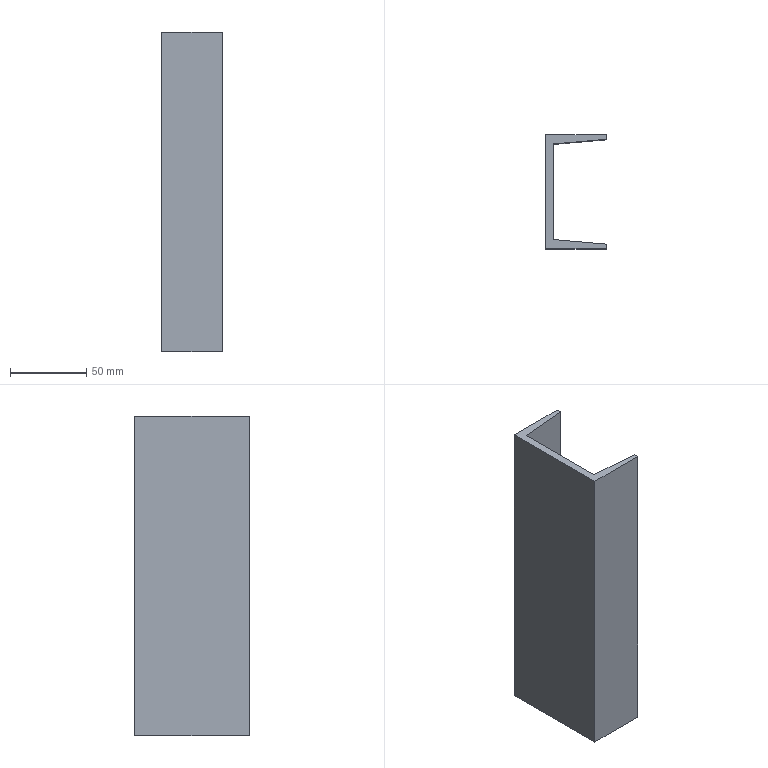Part | STEP file | BCC3 H13_7 | 1 solid | 10 faces | box 40 x 75 x 210 mm | volume 145356 mm3 | plane 10
STEP:
#1=CARTESIAN_POINT('',(0.,0.,0.));
#2=DIRECTION('',(0.,0.,1.));
#3=DIRECTION('',(1.,0.,0.));
#4=AXIS2_PLACEMENT_3D('',#1,#2,#3);
#5=CARTESIAN_POINT('',(40.,37.5,-105.));
#6=VERTEX_POINT('',#5);
#7=CARTESIAN_POINT('',(0.,37.5,-105.));
#8=VERTEX_POINT('',#7);
#9=CARTESIAN_POINT('',(40.,37.5,-105.));
#10=DIRECTION('',(-1.,0.,0.));
#11=VECTOR('',#10,1.);
#12=LINE('',#9,#11);
#13=CARTESIAN_POINT('',(40.,37.5,105.));
#14=DIRECTION('',(0.,-1.,0.));
#15=DIRECTION('',(0.,0.,-1.));
#16=AXIS2_PLACEMENT_3D('',#13,#14,#15);
#17=PLANE('',#16);
#18=CARTESIAN_POINT('',(210.,0.));
#19=DIRECTION('',(0.,-1.));
#20=VECTOR('',#19,1.);
#21=LINE('',#18,#20);
#22=(GEOMETRIC_REPRESENTATION_CONTEXT(2)PARAMETRIC_REPRESENTATION_CONTEXT()REPRESENTATION_CONTEXT('',''));
#23=DEFINITIONAL_REPRESENTATION('',(#21),#22);
#24=PCURVE('',#17,#23);
#25=CARTESIAN_POINT('',(0.,0.,-105.));
#26=DIRECTION('',(0.,0.,1.));
#27=DIRECTION('',(1.,0.,0.));
#28=AXIS2_PLACEMENT_3D('',#25,#26,#27);
#29=PLANE('',#28);
#30=CARTESIAN_POINT('',(40.,37.5));
#31=DIRECTION('',(-1.,0.));
#32=VECTOR('',#31,1.);
#33=LINE('',#30,#32);
#34=(GEOMETRIC_REPRESENTATION_CONTEXT(2)PARAMETRIC_REPRESENTATION_CONTEXT()REPRESENTATION_CONTEXT('',''));
#35=DEFINITIONAL_REPRESENTATION('',(#33),#34);
#36=PCURVE('',#29,#35);
#37=SURFACE_CURVE('',#12,(#24,#36),.PCURVE_S1.);
#38=EDGE_CURVE('',#6,#8,#37,.T.);
#39=ORIENTED_EDGE('',*,*,#38,.T.);
#40=CARTESIAN_POINT('',(0.,37.5,105.));
#41=VERTEX_POINT('',#40);
#42=CARTESIAN_POINT('',(0.,37.5,105.));
#43=DIRECTION('',(0.,0.,-1.));
#44=VECTOR('',#43,1.);
#45=LINE('',#42,#44);
#46=CARTESIAN_POINT('',(0.,-40.));
#47=DIRECTION('',(1.,0.));
#48=VECTOR('',#47,1.);
#49=LINE('',#46,#48);
#50=(GEOMETRIC_REPRESENTATION_CONTEXT(2)PARAMETRIC_REPRESENTATION_CONTEXT()REPRESENTATION_CONTEXT('',''));
#51=DEFINITIONAL_REPRESENTATION('',(#49),#50);
#52=PCURVE('',#17,#51);
#53=CARTESIAN_POINT('',(0.,37.5,105.));
#54=DIRECTION('',(1.,0.,0.));
#55=DIRECTION('',(0.,0.,-1.));
#56=AXIS2_PLACEMENT_3D('',#53,#54,#55);
#57=PLANE('',#56);
#58=CARTESIAN_POINT('',(0.,0.));
#59=DIRECTION('',(1.,0.));
#60=VECTOR('',#59,1.);
#61=LINE('',#58,#60);
#62=(GEOMETRIC_REPRESENTATION_CONTEXT(2)PARAMETRIC_REPRESENTATION_CONTEXT()REPRESENTATION_CONTEXT('',''));
#63=DEFINITIONAL_REPRESENTATION('',(#61),#62);
#64=PCURVE('',#57,#63);
#65=SURFACE_CURVE('',#45,(#52,#64),.PCURVE_S1.);
#66=EDGE_CURVE('',#41,#8,#65,.T.);
#67=ORIENTED_EDGE('',*,*,#66,.F.);
#68=CARTESIAN_POINT('',(40.,37.5,105.));
#69=VERTEX_POINT('',#68);
#70=CARTESIAN_POINT('',(40.,37.5,105.));
#71=DIRECTION('',(-1.,0.,0.));
#72=VECTOR('',#71,1.);
#73=LINE('',#70,#72);
#74=CARTESIAN_POINT('',(0.,0.));
#75=DIRECTION('',(0.,-1.));
#76=VECTOR('',#75,1.);
#77=LINE('',#74,#76);
#78=(GEOMETRIC_REPRESENTATION_CONTEXT(2)PARAMETRIC_REPRESENTATION_CONTEXT()REPRESENTATION_CONTEXT('',''));
#79=DEFINITIONAL_REPRESENTATION('',(#77),#78);
#80=PCURVE('',#17,#79);
#81=CARTESIAN_POINT('',(0.,0.,105.));
#82=DIRECTION('',(0.,0.,1.));
#83=DIRECTION('',(1.,0.,0.));
#84=AXIS2_PLACEMENT_3D('',#81,#82,#83);
#85=PLANE('',#84);
#86=CARTESIAN_POINT('',(40.,37.5));
#87=DIRECTION('',(-1.,0.));
#88=VECTOR('',#87,1.);
#89=LINE('',#86,#88);
#90=(GEOMETRIC_REPRESENTATION_CONTEXT(2)PARAMETRIC_REPRESENTATION_CONTEXT()REPRESENTATION_CONTEXT('',''));
#91=DEFINITIONAL_REPRESENTATION('',(#89),#90);
#92=PCURVE('',#85,#91);
#93=SURFACE_CURVE('',#73,(#80,#92),.PCURVE_S1.);
#94=EDGE_CURVE('',#69,#41,#93,.T.);
#95=ORIENTED_EDGE('',*,*,#94,.F.);
#96=CARTESIAN_POINT('',(40.,37.5,105.));
#97=DIRECTION('',(0.,0.,-1.));
#98=VECTOR('',#97,1.);
#99=LINE('',#96,#98);
#100=CARTESIAN_POINT('',(0.,0.));
#101=DIRECTION('',(1.,0.));
#102=VECTOR('',#101,1.);
#103=LINE('',#100,#102);
#104=(GEOMETRIC_REPRESENTATION_CONTEXT(2)PARAMETRIC_REPRESENTATION_CONTEXT()REPRESENTATION_CONTEXT('',''));
#105=DEFINITIONAL_REPRESENTATION('',(#103),#104);
#106=PCURVE('',#17,#105);
#107=CARTESIAN_POINT('',(40.,34.5,105.));
#108=DIRECTION('',(-1.,0.,0.));
#109=DIRECTION('',(0.,0.,1.));
#110=AXIS2_PLACEMENT_3D('',#107,#108,#109);
#111=PLANE('',#110);
#112=CARTESIAN_POINT('',(0.,3.));
#113=DIRECTION('',(-1.,0.));
#114=VECTOR('',#113,1.);
#115=LINE('',#112,#114);
#116=(GEOMETRIC_REPRESENTATION_CONTEXT(2)PARAMETRIC_REPRESENTATION_CONTEXT()REPRESENTATION_CONTEXT('',''));
#117=DEFINITIONAL_REPRESENTATION('',(#115),#116);
#118=PCURVE('',#111,#117);
#119=SURFACE_CURVE('',#99,(#106,#118),.PCURVE_S1.);
#120=EDGE_CURVE('',#69,#6,#119,.T.);
#121=ORIENTED_EDGE('',*,*,#120,.T.);
#122=EDGE_LOOP('',(#39,#67,#95,#121));
#123=FACE_BOUND('',#122,.T.);
#124=ADVANCED_FACE('',(#123),#17,.F.);
#125=CARTESIAN_POINT('',(0.,-37.5,-105.));
#126=VERTEX_POINT('',#125);
#127=CARTESIAN_POINT('',(0.,37.5,-105.));
#128=DIRECTION('',(0.,-1.,0.));
#129=VECTOR('',#128,1.);
#130=LINE('',#127,#129);
#131=CARTESIAN_POINT('',(210.,0.));
#132=DIRECTION('',(0.,-1.));
#133=VECTOR('',#132,1.);
#134=LINE('',#131,#133);
#135=(GEOMETRIC_REPRESENTATION_CONTEXT(2)PARAMETRIC_REPRESENTATION_CONTEXT()REPRESENTATION_CONTEXT('',''));
#136=DEFINITIONAL_REPRESENTATION('',(#134),#135);
#137=PCURVE('',#57,#136);
#138=CARTESIAN_POINT('',(0.,37.5));
#139=DIRECTION('',(0.,-1.));
#140=VECTOR('',#139,1.);
#141=LINE('',#138,#140);
#142=(GEOMETRIC_REPRESENTATION_CONTEXT(2)PARAMETRIC_REPRESENTATION_CONTEXT()REPRESENTATION_CONTEXT('',''));
#143=DEFINITIONAL_REPRESENTATION('',(#141),#142);
#144=PCURVE('',#29,#143);
#145=SURFACE_CURVE('',#130,(#137,#144),.PCURVE_S1.);
#146=EDGE_CURVE('',#8,#126,#145,.T.);
#147=ORIENTED_EDGE('',*,*,#146,.T.);
#148=CARTESIAN_POINT('',(0.,-37.5,105.));
#149=VERTEX_POINT('',#148);
#150=CARTESIAN_POINT('',(0.,-37.5,105.));
#151=DIRECTION('',(0.,0.,-1.));
#152=VECTOR('',#151,1.);
#153=LINE('',#150,#152);
#154=CARTESIAN_POINT('',(0.,-75.));
#155=DIRECTION('',(1.,0.));
#156=VECTOR('',#155,1.);
#157=LINE('',#154,#156);
#158=(GEOMETRIC_REPRESENTATION_CONTEXT(2)PARAMETRIC_REPRESENTATION_CONTEXT()REPRESENTATION_CONTEXT('',''));
#159=DEFINITIONAL_REPRESENTATION('',(#157),#158);
#160=PCURVE('',#57,#159);
#161=CARTESIAN_POINT('',(0.,-37.5,105.));
#162=DIRECTION('',(0.,1.,0.));
#163=DIRECTION('',(0.,0.,1.));
#164=AXIS2_PLACEMENT_3D('',#161,#162,#163);
#165=PLANE('',#164);
#166=CARTESIAN_POINT('',(0.,0.));
#167=DIRECTION('',(-1.,0.));
#168=VECTOR('',#167,1.);
#169=LINE('',#166,#168);
#170=(GEOMETRIC_REPRESENTATION_CONTEXT(2)PARAMETRIC_REPRESENTATION_CONTEXT()REPRESENTATION_CONTEXT('',''));
#171=DEFINITIONAL_REPRESENTATION('',(#169),#170);
#172=PCURVE('',#165,#171);
#173=SURFACE_CURVE('',#153,(#160,#172),.PCURVE_S1.);
#174=EDGE_CURVE('',#149,#126,#173,.T.);
#175=ORIENTED_EDGE('',*,*,#174,.F.);
#176=CARTESIAN_POINT('',(0.,37.5,105.));
#177=DIRECTION('',(0.,-1.,0.));
#178=VECTOR('',#177,1.);
#179=LINE('',#176,#178);
#180=CARTESIAN_POINT('',(0.,0.));
#181=DIRECTION('',(0.,-1.));
#182=VECTOR('',#181,1.);
#183=LINE('',#180,#182);
#184=(GEOMETRIC_REPRESENTATION_CONTEXT(2)PARAMETRIC_REPRESENTATION_CONTEXT()REPRESENTATION_CONTEXT('',''));
#185=DEFINITIONAL_REPRESENTATION('',(#183),#184);
#186=PCURVE('',#57,#185);
#187=CARTESIAN_POINT('',(0.,37.5));
#188=DIRECTION('',(0.,-1.));
#189=VECTOR('',#188,1.);
#190=LINE('',#187,#189);
#191=(GEOMETRIC_REPRESENTATION_CONTEXT(2)PARAMETRIC_REPRESENTATION_CONTEXT()REPRESENTATION_CONTEXT('',''));
#192=DEFINITIONAL_REPRESENTATION('',(#190),#191);
#193=PCURVE('',#85,#192);
#194=SURFACE_CURVE('',#179,(#186,#193),.PCURVE_S1.);
#195=EDGE_CURVE('',#41,#149,#194,.T.);
#196=ORIENTED_EDGE('',*,*,#195,.F.);
#197=ORIENTED_EDGE('',*,*,#66,.T.);
#198=EDGE_LOOP('',(#147,#175,#196,#197));
#199=FACE_BOUND('',#198,.T.);
#200=ADVANCED_FACE('',(#199),#57,.F.);
#201=CARTESIAN_POINT('',(40.,-37.5,-105.));
#202=VERTEX_POINT('',#201);
#203=CARTESIAN_POINT('',(0.,-37.5,-105.));
#204=DIRECTION('',(1.,0.,0.));
#205=VECTOR('',#204,1.);
#206=LINE('',#203,#205);
#207=CARTESIAN_POINT('',(-210.,0.));
#208=DIRECTION('',(0.,1.));
#209=VECTOR('',#208,1.);
#210=LINE('',#207,#209);
#211=(GEOMETRIC_REPRESENTATION_CONTEXT(2)PARAMETRIC_REPRESENTATION_CONTEXT()REPRESENTATION_CONTEXT('',''));
#212=DEFINITIONAL_REPRESENTATION('',(#210),#211);
#213=PCURVE('',#165,#212);
#214=CARTESIAN_POINT('',(0.,-37.5));
#215=DIRECTION('',(1.,0.));
#216=VECTOR('',#215,1.);
#217=LINE('',#214,#216);
#218=(GEOMETRIC_REPRESENTATION_CONTEXT(2)PARAMETRIC_REPRESENTATION_CONTEXT()REPRESENTATION_CONTEXT('',''));
#219=DEFINITIONAL_REPRESENTATION('',(#217),#218);
#220=PCURVE('',#29,#219);
#221=SURFACE_CURVE('',#206,(#213,#220),.PCURVE_S1.);
#222=EDGE_CURVE('',#126,#202,#221,.T.);
#223=ORIENTED_EDGE('',*,*,#222,.T.);
#224=CARTESIAN_POINT('',(40.,-37.5,105.));
#225=VERTEX_POINT('',#224);
#226=CARTESIAN_POINT('',(40.,-37.5,105.));
#227=DIRECTION('',(0.,0.,-1.));
#228=VECTOR('',#227,1.);
#229=LINE('',#226,#228);
#230=CARTESIAN_POINT('',(0.,40.));
#231=DIRECTION('',(-1.,0.));
#232=VECTOR('',#231,1.);
#233=LINE('',#230,#232);
#234=(GEOMETRIC_REPRESENTATION_CONTEXT(2)PARAMETRIC_REPRESENTATION_CONTEXT()REPRESENTATION_CONTEXT('',''));
#235=DEFINITIONAL_REPRESENTATION('',(#233),#234);
#236=PCURVE('',#165,#235);
#237=CARTESIAN_POINT('',(40.,-37.5,105.));
#238=DIRECTION('',(-1.,0.,0.));
#239=DIRECTION('',(0.,0.,1.));
#240=AXIS2_PLACEMENT_3D('',#237,#238,#239);
#241=PLANE('',#240);
#242=CARTESIAN_POINT('',(0.,0.));
#243=DIRECTION('',(-1.,0.));
#244=VECTOR('',#243,1.);
#245=LINE('',#242,#244);
#246=(GEOMETRIC_REPRESENTATION_CONTEXT(2)PARAMETRIC_REPRESENTATION_CONTEXT()REPRESENTATION_CONTEXT('',''));
#247=DEFINITIONAL_REPRESENTATION('',(#245),#246);
#248=PCURVE('',#241,#247);
#249=SURFACE_CURVE('',#229,(#236,#248),.PCURVE_S1.);
#250=EDGE_CURVE('',#225,#202,#249,.T.);
#251=ORIENTED_EDGE('',*,*,#250,.F.);
#252=CARTESIAN_POINT('',(0.,-37.5,105.));
#253=DIRECTION('',(1.,0.,0.));
#254=VECTOR('',#253,1.);
#255=LINE('',#252,#254);
#256=CARTESIAN_POINT('',(0.,0.));
#257=DIRECTION('',(0.,1.));
#258=VECTOR('',#257,1.);
#259=LINE('',#256,#258);
#260=(GEOMETRIC_REPRESENTATION_CONTEXT(2)PARAMETRIC_REPRESENTATION_CONTEXT()REPRESENTATION_CONTEXT('',''));
#261=DEFINITIONAL_REPRESENTATION('',(#259),#260);
#262=PCURVE('',#165,#261);
#263=CARTESIAN_POINT('',(0.,-37.5));
#264=DIRECTION('',(1.,0.));
#265=VECTOR('',#264,1.);
#266=LINE('',#263,#265);
#267=(GEOMETRIC_REPRESENTATION_CONTEXT(2)PARAMETRIC_REPRESENTATION_CONTEXT()REPRESENTATION_CONTEXT('',''));
#268=DEFINITIONAL_REPRESENTATION('',(#266),#267);
#269=PCURVE('',#85,#268);
#270=SURFACE_CURVE('',#255,(#262,#269),.PCURVE_S1.);
#271=EDGE_CURVE('',#149,#225,#270,.T.);
#272=ORIENTED_EDGE('',*,*,#271,.F.);
#273=ORIENTED_EDGE('',*,*,#174,.T.);
#274=EDGE_LOOP('',(#223,#251,#272,#273));
#275=FACE_BOUND('',#274,.T.);
#276=ADVANCED_FACE('',(#275),#165,.F.);
#277=CARTESIAN_POINT('',(40.,-34.5,-105.));
#278=VERTEX_POINT('',#277);
#279=CARTESIAN_POINT('',(40.,-37.5,-105.));
#280=DIRECTION('',(0.,1.,0.));
#281=VECTOR('',#280,1.);
#282=LINE('',#279,#281);
#283=CARTESIAN_POINT('',(-210.,0.));
#284=DIRECTION('',(0.,1.));
#285=VECTOR('',#284,1.);
#286=LINE('',#283,#285);
#287=(GEOMETRIC_REPRESENTATION_CONTEXT(2)PARAMETRIC_REPRESENTATION_CONTEXT()REPRESENTATION_CONTEXT('',''));
#288=DEFINITIONAL_REPRESENTATION('',(#286),#287);
#289=PCURVE('',#241,#288);
#290=CARTESIAN_POINT('',(40.,-37.5));
#291=DIRECTION('',(0.,1.));
#292=VECTOR('',#291,1.);
#293=LINE('',#290,#292);
#294=(GEOMETRIC_REPRESENTATION_CONTEXT(2)PARAMETRIC_REPRESENTATION_CONTEXT()REPRESENTATION_CONTEXT('',''));
#295=DEFINITIONAL_REPRESENTATION('',(#293),#294);
#296=PCURVE('',#29,#295);
#297=SURFACE_CURVE('',#282,(#289,#296),.PCURVE_S1.);
#298=EDGE_CURVE('',#202,#278,#297,.T.);
#299=ORIENTED_EDGE('',*,*,#298,.T.);
#300=CARTESIAN_POINT('',(40.,-34.5,105.));
#301=VERTEX_POINT('',#300);
#302=CARTESIAN_POINT('',(40.,-34.5,105.));
#303=DIRECTION('',(0.,0.,-1.));
#304=VECTOR('',#303,1.);
#305=LINE('',#302,#304);
#306=CARTESIAN_POINT('',(0.,3.));
#307=DIRECTION('',(-1.,0.));
#308=VECTOR('',#307,1.);
#309=LINE('',#306,#308);
#310=(GEOMETRIC_REPRESENTATION_CONTEXT(2)PARAMETRIC_REPRESENTATION_CONTEXT()REPRESENTATION_CONTEXT('',''));
#311=DEFINITIONAL_REPRESENTATION('',(#309),#310);
#312=PCURVE('',#241,#311);
#313=CARTESIAN_POINT('',(40.,-34.5,105.));
#314=DIRECTION('',(-0.08716,-0.9962,0.));
#315=DIRECTION('',(0.9962,-0.08716,0.));
#316=AXIS2_PLACEMENT_3D('',#313,#314,#315);
#317=PLANE('',#316);
#318=CARTESIAN_POINT('',(0.,0.));
#319=DIRECTION('',(0.,-1.));
#320=VECTOR('',#319,1.);
#321=LINE('',#318,#320);
#322=(GEOMETRIC_REPRESENTATION_CONTEXT(2)PARAMETRIC_REPRESENTATION_CONTEXT()REPRESENTATION_CONTEXT('',''));
#323=DEFINITIONAL_REPRESENTATION('',(#321),#322);
#324=PCURVE('',#317,#323);
#325=SURFACE_CURVE('',#305,(#312,#324),.PCURVE_S1.);
#326=EDGE_CURVE('',#301,#278,#325,.T.);
#327=ORIENTED_EDGE('',*,*,#326,.F.);
#328=CARTESIAN_POINT('',(40.,-37.5,105.));
#329=DIRECTION('',(0.,1.,0.));
#330=VECTOR('',#329,1.);
#331=LINE('',#328,#330);
#332=CARTESIAN_POINT('',(0.,0.));
#333=DIRECTION('',(0.,1.));
#334=VECTOR('',#333,1.);
#335=LINE('',#332,#334);
#336=(GEOMETRIC_REPRESENTATION_CONTEXT(2)PARAMETRIC_REPRESENTATION_CONTEXT()REPRESENTATION_CONTEXT('',''));
#337=DEFINITIONAL_REPRESENTATION('',(#335),#336);
#338=PCURVE('',#241,#337);
#339=CARTESIAN_POINT('',(40.,-37.5));
#340=DIRECTION('',(0.,1.));
#341=VECTOR('',#340,1.);
#342=LINE('',#339,#341);
#343=(GEOMETRIC_REPRESENTATION_CONTEXT(2)PARAMETRIC_REPRESENTATION_CONTEXT()REPRESENTATION_CONTEXT('',''));
#344=DEFINITIONAL_REPRESENTATION('',(#342),#343);
#345=PCURVE('',#85,#344);
#346=SURFACE_CURVE('',#331,(#338,#345),.PCURVE_S1.);
#347=EDGE_CURVE('',#225,#301,#346,.T.);
#348=ORIENTED_EDGE('',*,*,#347,.F.);
#349=ORIENTED_EDGE('',*,*,#250,.T.);
#350=EDGE_LOOP('',(#299,#327,#348,#349));
#351=FACE_BOUND('',#350,.T.);
#352=ADVANCED_FACE('',(#351),#241,.F.);
#353=CARTESIAN_POINT('',(5.,-31.438,-105.));
#354=VERTEX_POINT('',#353);
#355=CARTESIAN_POINT('',(40.,-34.5,-105.));
#356=DIRECTION('',(-0.9962,0.08716,0.));
#357=VECTOR('',#356,1.);
#358=LINE('',#355,#357);
#359=CARTESIAN_POINT('',(0.,-210.));
#360=DIRECTION('',(-1.,0.));
#361=VECTOR('',#360,1.);
#362=LINE('',#359,#361);
#363=(GEOMETRIC_REPRESENTATION_CONTEXT(2)PARAMETRIC_REPRESENTATION_CONTEXT()REPRESENTATION_CONTEXT('',''));
#364=DEFINITIONAL_REPRESENTATION('',(#362),#363);
#365=PCURVE('',#317,#364);
#366=CARTESIAN_POINT('',(40.,-34.5));
#367=DIRECTION('',(-0.9962,0.08716));
#368=VECTOR('',#367,1.);
#369=LINE('',#366,#368);
#370=(GEOMETRIC_REPRESENTATION_CONTEXT(2)PARAMETRIC_REPRESENTATION_CONTEXT()REPRESENTATION_CONTEXT('',''));
#371=DEFINITIONAL_REPRESENTATION('',(#369),#370);
#372=PCURVE('',#29,#371);
#373=SURFACE_CURVE('',#358,(#365,#372),.PCURVE_S1.);
#374=EDGE_CURVE('',#278,#354,#373,.T.);
#375=ORIENTED_EDGE('',*,*,#374,.T.);
#376=CARTESIAN_POINT('',(5.,-31.438,105.));
#377=VERTEX_POINT('',#376);
#378=CARTESIAN_POINT('',(5.,-31.438,105.));
#379=DIRECTION('',(0.,0.,-1.));
#380=VECTOR('',#379,1.);
#381=LINE('',#378,#380);
#382=CARTESIAN_POINT('',(-35.134,0.));
#383=DIRECTION('',(0.,-1.));
#384=VECTOR('',#383,1.);
#385=LINE('',#382,#384);
#386=(GEOMETRIC_REPRESENTATION_CONTEXT(2)PARAMETRIC_REPRESENTATION_CONTEXT()REPRESENTATION_CONTEXT('',''));
#387=DEFINITIONAL_REPRESENTATION('',(#385),#386);
#388=PCURVE('',#317,#387);
#389=CARTESIAN_POINT('',(5.,-31.438,105.));
#390=DIRECTION('',(-1.,0.,0.));
#391=DIRECTION('',(0.,0.,1.));
#392=AXIS2_PLACEMENT_3D('',#389,#390,#391);
#393=PLANE('',#392);
#394=CARTESIAN_POINT('',(0.,0.));
#395=DIRECTION('',(-1.,0.));
#396=VECTOR('',#395,1.);
#397=LINE('',#394,#396);
#398=(GEOMETRIC_REPRESENTATION_CONTEXT(2)PARAMETRIC_REPRESENTATION_CONTEXT()REPRESENTATION_CONTEXT('',''));
#399=DEFINITIONAL_REPRESENTATION('',(#397),#398);
#400=PCURVE('',#393,#399);
#401=SURFACE_CURVE('',#381,(#388,#400),.PCURVE_S1.);
#402=EDGE_CURVE('',#377,#354,#401,.T.);
#403=ORIENTED_EDGE('',*,*,#402,.F.);
#404=CARTESIAN_POINT('',(40.,-34.5,105.));
#405=DIRECTION('',(-0.9962,0.08716,0.));
#406=VECTOR('',#405,1.);
#407=LINE('',#404,#406);
#408=CARTESIAN_POINT('',(0.,0.));
#409=DIRECTION('',(-1.,0.));
#410=VECTOR('',#409,1.);
#411=LINE('',#408,#410);
#412=(GEOMETRIC_REPRESENTATION_CONTEXT(2)PARAMETRIC_REPRESENTATION_CONTEXT()REPRESENTATION_CONTEXT('',''));
#413=DEFINITIONAL_REPRESENTATION('',(#411),#412);
#414=PCURVE('',#317,#413);
#415=CARTESIAN_POINT('',(40.,-34.5));
#416=DIRECTION('',(-0.9962,0.08716));
#417=VECTOR('',#416,1.);
#418=LINE('',#415,#417);
#419=(GEOMETRIC_REPRESENTATION_CONTEXT(2)PARAMETRIC_REPRESENTATION_CONTEXT()REPRESENTATION_CONTEXT('',''));
#420=DEFINITIONAL_REPRESENTATION('',(#418),#419);
#421=PCURVE('',#85,#420);
#422=SURFACE_CURVE('',#407,(#414,#421),.PCURVE_S1.);
#423=EDGE_CURVE('',#301,#377,#422,.T.);
#424=ORIENTED_EDGE('',*,*,#423,.F.);
#425=ORIENTED_EDGE('',*,*,#326,.T.);
#426=EDGE_LOOP('',(#375,#403,#424,#425));
#427=FACE_BOUND('',#426,.T.);
#428=ADVANCED_FACE('',(#427),#317,.F.);
#429=CARTESIAN_POINT('',(5.,31.438,-105.));
#430=VERTEX_POINT('',#429);
#431=CARTESIAN_POINT('',(5.,-31.438,-105.));
#432=DIRECTION('',(0.,1.,0.));
#433=VECTOR('',#432,1.);
#434=LINE('',#431,#433);
#435=CARTESIAN_POINT('',(-210.,0.));
#436=DIRECTION('',(0.,1.));
#437=VECTOR('',#436,1.);
#438=LINE('',#435,#437);
#439=(GEOMETRIC_REPRESENTATION_CONTEXT(2)PARAMETRIC_REPRESENTATION_CONTEXT()REPRESENTATION_CONTEXT('',''));
#440=DEFINITIONAL_REPRESENTATION('',(#438),#439);
#441=PCURVE('',#393,#440);
#442=CARTESIAN_POINT('',(5.,-31.438));
#443=DIRECTION('',(0.,1.));
#444=VECTOR('',#443,1.);
#445=LINE('',#442,#444);
#446=(GEOMETRIC_REPRESENTATION_CONTEXT(2)PARAMETRIC_REPRESENTATION_CONTEXT()REPRESENTATION_CONTEXT('',''));
#447=DEFINITIONAL_REPRESENTATION('',(#445),#446);
#448=PCURVE('',#29,#447);
#449=SURFACE_CURVE('',#434,(#441,#448),.PCURVE_S1.);
#450=EDGE_CURVE('',#354,#430,#449,.T.);
#451=ORIENTED_EDGE('',*,*,#450,.T.);
#452=CARTESIAN_POINT('',(5.,31.438,105.));
#453=VERTEX_POINT('',#452);
#454=CARTESIAN_POINT('',(5.,31.438,105.));
#455=DIRECTION('',(0.,0.,-1.));
#456=VECTOR('',#455,1.);
#457=LINE('',#454,#456);
#458=CARTESIAN_POINT('',(0.,62.876));
#459=DIRECTION('',(-1.,0.));
#460=VECTOR('',#459,1.);
#461=LINE('',#458,#460);
#462=(GEOMETRIC_REPRESENTATION_CONTEXT(2)PARAMETRIC_REPRESENTATION_CONTEXT()REPRESENTATION_CONTEXT('',''));
#463=DEFINITIONAL_REPRESENTATION('',(#461),#462);
#464=PCURVE('',#393,#463);
#465=CARTESIAN_POINT('',(5.,31.438,105.));
#466=DIRECTION('',(-0.08716,0.9962,0.));
#467=DIRECTION('',(-0.9962,-0.08716,0.));
#468=AXIS2_PLACEMENT_3D('',#465,#466,#467);
#469=PLANE('',#468);
#470=CARTESIAN_POINT('',(0.,0.));
#471=DIRECTION('',(0.,-1.));
#472=VECTOR('',#471,1.);
#473=LINE('',#470,#472);
#474=(GEOMETRIC_REPRESENTATION_CONTEXT(2)PARAMETRIC_REPRESENTATION_CONTEXT()REPRESENTATION_CONTEXT('',''));
#475=DEFINITIONAL_REPRESENTATION('',(#473),#474);
#476=PCURVE('',#469,#475);
#477=SURFACE_CURVE('',#457,(#464,#476),.PCURVE_S1.);
#478=EDGE_CURVE('',#453,#430,#477,.T.);
#479=ORIENTED_EDGE('',*,*,#478,.F.);
#480=CARTESIAN_POINT('',(5.,-31.438,105.));
#481=DIRECTION('',(0.,1.,0.));
#482=VECTOR('',#481,1.);
#483=LINE('',#480,#482);
#484=CARTESIAN_POINT('',(0.,0.));
#485=DIRECTION('',(0.,1.));
#486=VECTOR('',#485,1.);
#487=LINE('',#484,#486);
#488=(GEOMETRIC_REPRESENTATION_CONTEXT(2)PARAMETRIC_REPRESENTATION_CONTEXT()REPRESENTATION_CONTEXT('',''));
#489=DEFINITIONAL_REPRESENTATION('',(#487),#488);
#490=PCURVE('',#393,#489);
#491=CARTESIAN_POINT('',(5.,-31.438));
#492=DIRECTION('',(0.,1.));
#493=VECTOR('',#492,1.);
#494=LINE('',#491,#493);
#495=(GEOMETRIC_REPRESENTATION_CONTEXT(2)PARAMETRIC_REPRESENTATION_CONTEXT()REPRESENTATION_CONTEXT('',''));
#496=DEFINITIONAL_REPRESENTATION('',(#494),#495);
#497=PCURVE('',#85,#496);
#498=SURFACE_CURVE('',#483,(#490,#497),.PCURVE_S1.);
#499=EDGE_CURVE('',#377,#453,#498,.T.);
#500=ORIENTED_EDGE('',*,*,#499,.F.);
#501=ORIENTED_EDGE('',*,*,#402,.T.);
#502=EDGE_LOOP('',(#451,#479,#500,#501));
#503=FACE_BOUND('',#502,.T.);
#504=ADVANCED_FACE('',(#503),#393,.F.);
#505=CARTESIAN_POINT('',(40.,34.5,-105.));
#506=VERTEX_POINT('',#505);
#507=CARTESIAN_POINT('',(5.,31.438,-105.));
#508=DIRECTION('',(0.9962,0.08716,0.));
#509=VECTOR('',#508,1.);
#510=LINE('',#507,#509);
#511=CARTESIAN_POINT('',(0.,-210.));
#512=DIRECTION('',(-1.,0.));
#513=VECTOR('',#512,1.);
#514=LINE('',#511,#513);
#515=(GEOMETRIC_REPRESENTATION_CONTEXT(2)PARAMETRIC_REPRESENTATION_CONTEXT()REPRESENTATION_CONTEXT('',''));
#516=DEFINITIONAL_REPRESENTATION('',(#514),#515);
#517=PCURVE('',#469,#516);
#518=CARTESIAN_POINT('',(5.,31.438));
#519=DIRECTION('',(0.9962,0.08716));
#520=VECTOR('',#519,1.);
#521=LINE('',#518,#520);
#522=(GEOMETRIC_REPRESENTATION_CONTEXT(2)PARAMETRIC_REPRESENTATION_CONTEXT()REPRESENTATION_CONTEXT('',''));
#523=DEFINITIONAL_REPRESENTATION('',(#521),#522);
#524=PCURVE('',#29,#523);
#525=SURFACE_CURVE('',#510,(#517,#524),.PCURVE_S1.);
#526=EDGE_CURVE('',#430,#506,#525,.T.);
#527=ORIENTED_EDGE('',*,*,#526,.T.);
#528=CARTESIAN_POINT('',(40.,34.5,105.));
#529=VERTEX_POINT('',#528);
#530=CARTESIAN_POINT('',(40.,34.5,105.));
#531=DIRECTION('',(0.,0.,-1.));
#532=VECTOR('',#531,1.);
#533=LINE('',#530,#532);
#534=CARTESIAN_POINT('',(-35.134,0.));
#535=DIRECTION('',(0.,-1.));
#536=VECTOR('',#535,1.);
#537=LINE('',#534,#536);
#538=(GEOMETRIC_REPRESENTATION_CONTEXT(2)PARAMETRIC_REPRESENTATION_CONTEXT()REPRESENTATION_CONTEXT('',''));
#539=DEFINITIONAL_REPRESENTATION('',(#537),#538);
#540=PCURVE('',#469,#539);
#541=CARTESIAN_POINT('',(0.,0.));
#542=DIRECTION('',(-1.,0.));
#543=VECTOR('',#542,1.);
#544=LINE('',#541,#543);
#545=(GEOMETRIC_REPRESENTATION_CONTEXT(2)PARAMETRIC_REPRESENTATION_CONTEXT()REPRESENTATION_CONTEXT('',''));
#546=DEFINITIONAL_REPRESENTATION('',(#544),#545);
#547=PCURVE('',#111,#546);
#548=SURFACE_CURVE('',#533,(#540,#547),.PCURVE_S1.);
#549=EDGE_CURVE('',#529,#506,#548,.T.);
#550=ORIENTED_EDGE('',*,*,#549,.F.);
#551=CARTESIAN_POINT('',(5.,31.438,105.));
#552=DIRECTION('',(0.9962,0.08716,0.));
#553=VECTOR('',#552,1.);
#554=LINE('',#551,#553);
#555=CARTESIAN_POINT('',(0.,0.));
#556=DIRECTION('',(-1.,0.));
#557=VECTOR('',#556,1.);
#558=LINE('',#555,#557);
#559=(GEOMETRIC_REPRESENTATION_CONTEXT(2)PARAMETRIC_REPRESENTATION_CONTEXT()REPRESENTATION_CONTEXT('',''));
#560=DEFINITIONAL_REPRESENTATION('',(#558),#559);
#561=PCURVE('',#469,#560);
#562=CARTESIAN_POINT('',(5.,31.438));
#563=DIRECTION('',(0.9962,0.08716));
#564=VECTOR('',#563,1.);
#565=LINE('',#562,#564);
#566=(GEOMETRIC_REPRESENTATION_CONTEXT(2)PARAMETRIC_REPRESENTATION_CONTEXT()REPRESENTATION_CONTEXT('',''));
#567=DEFINITIONAL_REPRESENTATION('',(#565),#566);
#568=PCURVE('',#85,#567);
#569=SURFACE_CURVE('',#554,(#561,#568),.PCURVE_S1.);
#570=EDGE_CURVE('',#453,#529,#569,.T.);
#571=ORIENTED_EDGE('',*,*,#570,.F.);
#572=ORIENTED_EDGE('',*,*,#478,.T.);
#573=EDGE_LOOP('',(#527,#550,#571,#572));
#574=FACE_BOUND('',#573,.T.);
#575=ADVANCED_FACE('',(#574),#469,.F.);
#576=CARTESIAN_POINT('',(40.,34.5,-105.));
#577=DIRECTION('',(0.,1.,0.));
#578=VECTOR('',#577,1.);
#579=LINE('',#576,#578);
#580=CARTESIAN_POINT('',(-210.,0.));
#581=DIRECTION('',(0.,1.));
#582=VECTOR('',#581,1.);
#583=LINE('',#580,#582);
#584=(GEOMETRIC_REPRESENTATION_CONTEXT(2)PARAMETRIC_REPRESENTATION_CONTEXT()REPRESENTATION_CONTEXT('',''));
#585=DEFINITIONAL_REPRESENTATION('',(#583),#584);
#586=PCURVE('',#111,#585);
#587=CARTESIAN_POINT('',(40.,34.5));
#588=DIRECTION('',(0.,1.));
#589=VECTOR('',#588,1.);
#590=LINE('',#587,#589);
#591=(GEOMETRIC_REPRESENTATION_CONTEXT(2)PARAMETRIC_REPRESENTATION_CONTEXT()REPRESENTATION_CONTEXT('',''));
#592=DEFINITIONAL_REPRESENTATION('',(#590),#591);
#593=PCURVE('',#29,#592);
#594=SURFACE_CURVE('',#579,(#586,#593),.PCURVE_S1.);
#595=EDGE_CURVE('',#506,#6,#594,.T.);
#596=ORIENTED_EDGE('',*,*,#595,.T.);
#597=ORIENTED_EDGE('',*,*,#120,.F.);
#598=CARTESIAN_POINT('',(40.,34.5,105.));
#599=DIRECTION('',(0.,1.,0.));
#600=VECTOR('',#599,1.);
#601=LINE('',#598,#600);
#602=CARTESIAN_POINT('',(0.,0.));
#603=DIRECTION('',(0.,1.));
#604=VECTOR('',#603,1.);
#605=LINE('',#602,#604);
#606=(GEOMETRIC_REPRESENTATION_CONTEXT(2)PARAMETRIC_REPRESENTATION_CONTEXT()REPRESENTATION_CONTEXT('',''));
#607=DEFINITIONAL_REPRESENTATION('',(#605),#606);
#608=PCURVE('',#111,#607);
#609=CARTESIAN_POINT('',(40.,34.5));
#610=DIRECTION('',(0.,1.));
#611=VECTOR('',#610,1.);
#612=LINE('',#609,#611);
#613=(GEOMETRIC_REPRESENTATION_CONTEXT(2)PARAMETRIC_REPRESENTATION_CONTEXT()REPRESENTATION_CONTEXT('',''));
#614=DEFINITIONAL_REPRESENTATION('',(#612),#613);
#615=PCURVE('',#85,#614);
#616=SURFACE_CURVE('',#601,(#608,#615),.PCURVE_S1.);
#617=EDGE_CURVE('',#529,#69,#616,.T.);
#618=ORIENTED_EDGE('',*,*,#617,.F.);
#619=ORIENTED_EDGE('',*,*,#549,.T.);
#620=EDGE_LOOP('',(#596,#597,#618,#619));
#621=FACE_BOUND('',#620,.T.);
#622=ADVANCED_FACE('',(#621),#111,.F.);
#623=ORIENTED_EDGE('',*,*,#94,.T.);
#624=ORIENTED_EDGE('',*,*,#195,.T.);
#625=ORIENTED_EDGE('',*,*,#271,.T.);
#626=ORIENTED_EDGE('',*,*,#347,.T.);
#627=ORIENTED_EDGE('',*,*,#423,.T.);
#628=ORIENTED_EDGE('',*,*,#499,.T.);
#629=ORIENTED_EDGE('',*,*,#570,.T.);
#630=ORIENTED_EDGE('',*,*,#617,.T.);
#631=EDGE_LOOP('',(#623,#624,#625,#626,#627,#628,#629,#630));
#632=FACE_BOUND('',#631,.T.);
#633=ADVANCED_FACE('',(#632),#85,.T.);
#634=ORIENTED_EDGE('',*,*,#38,.F.);
#635=ORIENTED_EDGE('',*,*,#595,.F.);
#636=ORIENTED_EDGE('',*,*,#526,.F.);
#637=ORIENTED_EDGE('',*,*,#450,.F.);
#638=ORIENTED_EDGE('',*,*,#374,.F.);
#639=ORIENTED_EDGE('',*,*,#298,.F.);
#640=ORIENTED_EDGE('',*,*,#222,.F.);
#641=ORIENTED_EDGE('',*,*,#146,.F.);
#642=EDGE_LOOP('',(#634,#635,#636,#637,#638,#639,#640,#641));
#643=FACE_BOUND('',#642,.T.);
#644=ADVANCED_FACE('',(#643),#29,.F.);
#645=CLOSED_SHELL('',(#124,#200,#276,#352,#428,#504,#575,#622,#633,#644));
#646=MANIFOLD_SOLID_BREP('',#645);
#647=(LENGTH_UNIT()NAMED_UNIT(*)SI_UNIT(.MILLI.,.METRE.));
#648=UNCERTAINTY_MEASURE_WITH_UNIT(LENGTH_MEASURE(0.0000001),#647,'','');
#649=(NAMED_UNIT(*)PLANE_ANGLE_UNIT()SI_UNIT($,.RADIAN.));
#650=(NAMED_UNIT(*)SI_UNIT($,.STERADIAN.)SOLID_ANGLE_UNIT());
#651=(GEOMETRIC_REPRESENTATION_CONTEXT(3)GLOBAL_UNCERTAINTY_ASSIGNED_CONTEXT((#648))GLOBAL_UNIT_ASSIGNED_CONTEXT((#647,#649,#650))REPRESENTATION_CONTEXT('',''));
#652=ADVANCED_BREP_SHAPE_REPRESENTATION('',(#4,#646),#651);